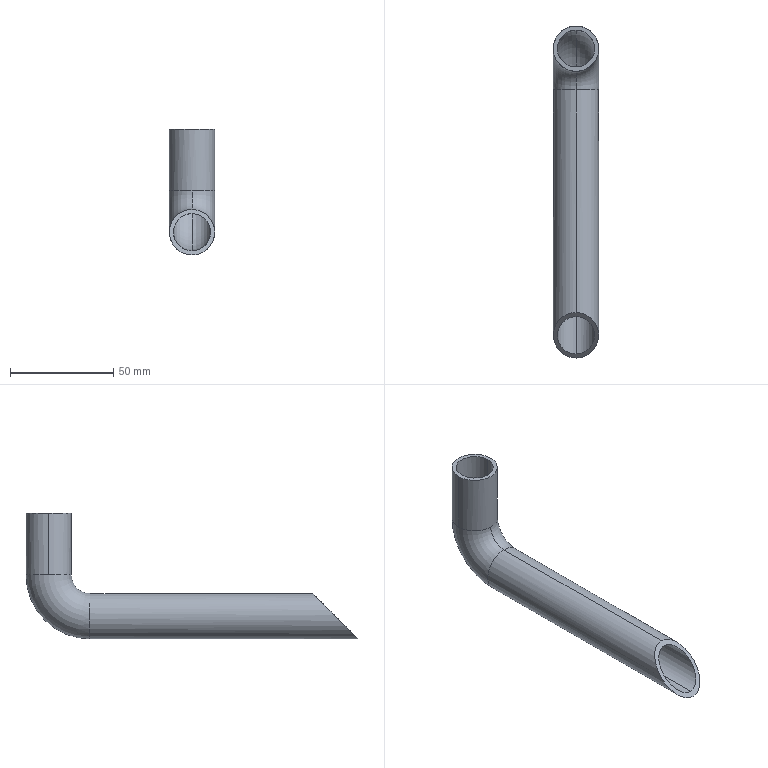Part | SolidWorks | features ICE 1, Sweep 1 | 1 solid | 14 faces | box 22 x 161 x 61 mm | volume 22672 mm3 | cylinder 8 | torus 4 | plane 2 | commonest cylinder face diameters 18 x4 22 x4
STEP:
#1=CARTESIAN_POINT('',(9.,0.,-30.));
#2=VERTEX_POINT('',#1);
#3=CARTESIAN_POINT('',(0.,9.,-30.));
#4=VERTEX_POINT('',#3);
#5=CARTESIAN_POINT('',(0.,0.,-30.));
#6=DIRECTION('',(0.,0.,1.));
#7=DIRECTION('',(1.,0.,0.));
#8=AXIS2_PLACEMENT_3D('',#5,#6,#7);
#9=CIRCLE('',#8,9.);
#10=EDGE_CURVE('',#2,#4,#9,.T.);
#11=ORIENTED_EDGE('',*,*,#10,.T.);
#12=CARTESIAN_POINT('',(0.,-20.,-59.));
#13=VERTEX_POINT('',#12);
#14=CARTESIAN_POINT('',(0.,-20.,-30.));
#15=DIRECTION('',(-1.,0.,0.));
#16=DIRECTION('',(0.,0.,1.));
#17=AXIS2_PLACEMENT_3D('',#14,#15,#16);
#18=CIRCLE('',#17,29.);
#19=EDGE_CURVE('',#4,#13,#18,.T.);
#20=ORIENTED_EDGE('',*,*,#19,.T.);
#21=CARTESIAN_POINT('',(0.,-20.,-41.));
#22=VERTEX_POINT('',#21);
#23=CARTESIAN_POINT('',(0.,-20.,-50.));
#24=DIRECTION('',(0.,1.,0.));
#25=DIRECTION('',(1.,0.,0.));
#26=AXIS2_PLACEMENT_3D('',#23,#24,#25);
#27=CIRCLE('',#26,9.);
#28=EDGE_CURVE('',#22,#13,#27,.T.);
#29=ORIENTED_EDGE('',*,*,#28,.F.);
#30=CARTESIAN_POINT('',(0.,-9.,-30.));
#31=VERTEX_POINT('',#30);
#32=CARTESIAN_POINT('',(0.,-20.,-30.));
#33=DIRECTION('',(-1.,0.,0.));
#34=DIRECTION('',(0.,0.,1.));
#35=AXIS2_PLACEMENT_3D('',#32,#33,#34);
#36=CIRCLE('',#35,11.);
#37=EDGE_CURVE('',#31,#22,#36,.T.);
#38=ORIENTED_EDGE('',*,*,#37,.F.);
#39=CARTESIAN_POINT('',(0.,0.,-30.));
#40=DIRECTION('',(0.,0.,1.));
#41=DIRECTION('',(1.,0.,0.));
#42=AXIS2_PLACEMENT_3D('',#39,#40,#41);
#43=CIRCLE('',#42,9.);
#44=EDGE_CURVE('',#31,#2,#43,.T.);
#45=ORIENTED_EDGE('',*,*,#44,.T.);
#46=EDGE_LOOP('',(#11,#20,#29,#38,#45));
#47=FACE_OUTER_BOUND('',#46,.T.);
#48=CARTESIAN_POINT('',(0.,-20.,-30.));
#49=DIRECTION('',(-1.,0.,0.));
#50=DIRECTION('',(0.,0.,1.));
#51=AXIS2_PLACEMENT_3D('',#48,#49,#50);
#52=TOROIDAL_SURFACE('',#51,20.,9.);
#53=ADVANCED_FACE('',(#47),#52,.F.);
#54=CARTESIAN_POINT('',(0.,11.,-30.));
#55=VERTEX_POINT('',#54);
#56=CARTESIAN_POINT('',(-11.,0.,-30.));
#57=VERTEX_POINT('',#56);
#58=CARTESIAN_POINT('',(0.,0.,-30.));
#59=DIRECTION('',(0.,0.,1.));
#60=DIRECTION('',(1.,0.,0.));
#61=AXIS2_PLACEMENT_3D('',#58,#59,#60);
#62=CIRCLE('',#61,11.);
#63=EDGE_CURVE('',#55,#57,#62,.T.);
#64=ORIENTED_EDGE('',*,*,#63,.F.);
#65=CARTESIAN_POINT('',(0.,-20.,-61.));
#66=VERTEX_POINT('',#65);
#67=CARTESIAN_POINT('',(0.,-20.,-30.));
#68=DIRECTION('',(-1.,0.,0.));
#69=DIRECTION('',(0.,0.,1.));
#70=AXIS2_PLACEMENT_3D('',#67,#68,#69);
#71=CIRCLE('',#70,31.);
#72=EDGE_CURVE('',#55,#66,#71,.T.);
#73=ORIENTED_EDGE('',*,*,#72,.T.);
#74=CARTESIAN_POINT('',(0.,-20.,-39.));
#75=VERTEX_POINT('',#74);
#76=CARTESIAN_POINT('',(0.,-20.,-50.));
#77=DIRECTION('',(0.,1.,0.));
#78=DIRECTION('',(1.,0.,0.));
#79=AXIS2_PLACEMENT_3D('',#76,#77,#78);
#80=CIRCLE('',#79,11.);
#81=EDGE_CURVE('',#66,#75,#80,.T.);
#82=ORIENTED_EDGE('',*,*,#81,.T.);
#83=CARTESIAN_POINT('',(0.,-11.,-30.));
#84=VERTEX_POINT('',#83);
#85=CARTESIAN_POINT('',(0.,-20.,-30.));
#86=DIRECTION('',(-1.,0.,0.));
#87=DIRECTION('',(0.,0.,1.));
#88=AXIS2_PLACEMENT_3D('',#85,#86,#87);
#89=CIRCLE('',#88,9.);
#90=EDGE_CURVE('',#84,#75,#89,.T.);
#91=ORIENTED_EDGE('',*,*,#90,.F.);
#92=CARTESIAN_POINT('',(0.,0.,-30.));
#93=DIRECTION('',(0.,0.,1.));
#94=DIRECTION('',(1.,0.,0.));
#95=AXIS2_PLACEMENT_3D('',#92,#93,#94);
#96=CIRCLE('',#95,11.);
#97=EDGE_CURVE('',#57,#84,#96,.T.);
#98=ORIENTED_EDGE('',*,*,#97,.F.);
#99=EDGE_LOOP('',(#64,#73,#82,#91,#98));
#100=FACE_OUTER_BOUND('',#99,.T.);
#101=CARTESIAN_POINT('',(0.,-20.,-30.));
#102=DIRECTION('',(-1.,0.,0.));
#103=DIRECTION('',(0.,0.,1.));
#104=AXIS2_PLACEMENT_3D('',#101,#102,#103);
#105=TOROIDAL_SURFACE('',#104,20.,11.);
#106=ADVANCED_FACE('',(#100),#105,.T.);
#107=CARTESIAN_POINT('',(11.,0.,-30.));
#108=VERTEX_POINT('',#107);
#109=CARTESIAN_POINT('',(0.,0.,-30.));
#110=DIRECTION('',(0.,0.,1.));
#111=DIRECTION('',(1.,0.,0.));
#112=AXIS2_PLACEMENT_3D('',#109,#110,#111);
#113=CIRCLE('',#112,11.);
#114=EDGE_CURVE('',#108,#55,#113,.T.);
#115=ORIENTED_EDGE('',*,*,#114,.T.);
#116=ORIENTED_EDGE('',*,*,#63,.T.);
#117=CARTESIAN_POINT('',(-11.,0.,0.));
#118=VERTEX_POINT('',#117);
#119=CARTESIAN_POINT('',(-11.,0.,-30.));
#120=DIRECTION('',(0.,0.,1.));
#121=VECTOR('',#120,1000.);
#122=LINE('',#119,#121);
#123=EDGE_CURVE('',#57,#118,#122,.T.);
#124=ORIENTED_EDGE('',*,*,#123,.T.);
#125=CARTESIAN_POINT('',(11.,0.,0.));
#126=VERTEX_POINT('',#125);
#127=CARTESIAN_POINT('',(0.,0.,0.));
#128=DIRECTION('',(0.,0.,1.));
#129=DIRECTION('',(1.,0.,0.));
#130=AXIS2_PLACEMENT_3D('',#127,#128,#129);
#131=CIRCLE('',#130,11.);
#132=EDGE_CURVE('',#126,#118,#131,.T.);
#133=ORIENTED_EDGE('',*,*,#132,.F.);
#134=CARTESIAN_POINT('',(11.,0.,-30.));
#135=DIRECTION('',(0.,0.,1.));
#136=VECTOR('',#135,1000.);
#137=LINE('',#134,#136);
#138=EDGE_CURVE('',#108,#126,#137,.T.);
#139=ORIENTED_EDGE('',*,*,#138,.F.);
#140=EDGE_LOOP('',(#115,#116,#124,#133,#139));
#141=FACE_OUTER_BOUND('',#140,.T.);
#142=CARTESIAN_POINT('',(0.,0.,-30.));
#143=DIRECTION('',(0.,0.,1.));
#144=DIRECTION('',(1.,0.,0.));
#145=AXIS2_PLACEMENT_3D('',#142,#143,#144);
#146=CYLINDRICAL_SURFACE('',#145,11.);
#147=ADVANCED_FACE('',(#141),#146,.T.);
#148=CARTESIAN_POINT('',(-9.,0.,-30.));
#149=VERTEX_POINT('',#148);
#150=CARTESIAN_POINT('',(0.,0.,-30.));
#151=DIRECTION('',(0.,0.,1.));
#152=DIRECTION('',(1.,0.,0.));
#153=AXIS2_PLACEMENT_3D('',#150,#151,#152);
#154=CIRCLE('',#153,9.);
#155=EDGE_CURVE('',#149,#31,#154,.T.);
#156=ORIENTED_EDGE('',*,*,#155,.F.);
#157=CARTESIAN_POINT('',(-9.,0.,0.));
#158=VERTEX_POINT('',#157);
#159=CARTESIAN_POINT('',(-9.,0.,-30.));
#160=DIRECTION('',(0.,0.,1.));
#161=VECTOR('',#160,1000.);
#162=LINE('',#159,#161);
#163=EDGE_CURVE('',#149,#158,#162,.T.);
#164=ORIENTED_EDGE('',*,*,#163,.T.);
#165=CARTESIAN_POINT('',(9.,0.,0.));
#166=VERTEX_POINT('',#165);
#167=CARTESIAN_POINT('',(0.,0.,0.));
#168=DIRECTION('',(0.,0.,1.));
#169=DIRECTION('',(1.,0.,0.));
#170=AXIS2_PLACEMENT_3D('',#167,#168,#169);
#171=CIRCLE('',#170,9.);
#172=EDGE_CURVE('',#158,#166,#171,.T.);
#173=ORIENTED_EDGE('',*,*,#172,.T.);
#174=CARTESIAN_POINT('',(9.,0.,-30.));
#175=DIRECTION('',(0.,0.,1.));
#176=VECTOR('',#175,1000.);
#177=LINE('',#174,#176);
#178=EDGE_CURVE('',#2,#166,#177,.T.);
#179=ORIENTED_EDGE('',*,*,#178,.F.);
#180=ORIENTED_EDGE('',*,*,#44,.F.);
#181=EDGE_LOOP('',(#156,#164,#173,#179,#180));
#182=FACE_OUTER_BOUND('',#181,.T.);
#183=CARTESIAN_POINT('',(0.,0.,-30.));
#184=DIRECTION('',(0.,0.,1.));
#185=DIRECTION('',(1.,0.,0.));
#186=AXIS2_PLACEMENT_3D('',#183,#184,#185);
#187=CYLINDRICAL_SURFACE('',#186,9.);
#188=ADVANCED_FACE('',(#182),#187,.F.);
#189=CARTESIAN_POINT('',(0.,-20.,-50.));
#190=DIRECTION('',(0.,1.,0.));
#191=DIRECTION('',(1.,0.,0.));
#192=AXIS2_PLACEMENT_3D('',#189,#190,#191);
#193=CIRCLE('',#192,9.);
#194=EDGE_CURVE('',#13,#22,#193,.T.);
#195=ORIENTED_EDGE('',*,*,#194,.T.);
#196=CARTESIAN_POINT('',(0.,-130.,-41.));
#197=VERTEX_POINT('',#196);
#198=CARTESIAN_POINT('',(0.,-20.,-41.));
#199=DIRECTION('',(0.,-1.,0.));
#200=VECTOR('',#199,1000.);
#201=LINE('',#198,#200);
#202=EDGE_CURVE('',#22,#197,#201,.T.);
#203=ORIENTED_EDGE('',*,*,#202,.T.);
#204=CARTESIAN_POINT('',(0.,-148.,-59.));
#205=VERTEX_POINT('',#204);
#206=CARTESIAN_POINT('',(0.,-148.,-59.));
#207=CARTESIAN_POINT('',(-18.,-148.,-59.));
#208=CARTESIAN_POINT('',(-18.,-130.,-41.));
#209=CARTESIAN_POINT('',(0.,-130.,-41.));
#210=(BOUNDED_CURVE()B_SPLINE_CURVE(3,(#206,#207,#208,#209),.UNSPECIFIED.,.F.,.T.)B_SPLINE_CURVE_WITH_KNOTS((4,4),(0.,3.142),.UNSPECIFIED.)CURVE()GEOMETRIC_REPRESENTATION_ITEM()RATIONAL_B_SPLINE_CURVE((1.,0.3333,0.3333,1.))REPRESENTATION_ITEM(''));
#211=EDGE_CURVE('',#205,#197,#210,.T.);
#212=ORIENTED_EDGE('',*,*,#211,.F.);
#213=CARTESIAN_POINT('',(0.,-20.,-59.));
#214=DIRECTION('',(0.,-1.,0.));
#215=VECTOR('',#214,1000.);
#216=LINE('',#213,#215);
#217=EDGE_CURVE('',#13,#205,#216,.T.);
#218=ORIENTED_EDGE('',*,*,#217,.F.);
#219=EDGE_LOOP('',(#195,#203,#212,#218));
#220=FACE_OUTER_BOUND('',#219,.T.);
#221=CARTESIAN_POINT('',(0.,-20.,-50.));
#222=DIRECTION('',(0.,-1.,0.));
#223=DIRECTION('',(0.,0.,-1.));
#224=AXIS2_PLACEMENT_3D('',#221,#222,#223);
#225=CYLINDRICAL_SURFACE('',#224,9.);
#226=ADVANCED_FACE('',(#220),#225,.F.);
#227=CARTESIAN_POINT('',(0.,-20.,-50.));
#228=DIRECTION('',(0.,1.,0.));
#229=DIRECTION('',(1.,0.,0.));
#230=AXIS2_PLACEMENT_3D('',#227,#228,#229);
#231=CIRCLE('',#230,11.);
#232=EDGE_CURVE('',#75,#66,#231,.T.);
#233=ORIENTED_EDGE('',*,*,#232,.F.);
#234=CARTESIAN_POINT('',(0.,-128.,-39.));
#235=VERTEX_POINT('',#234);
#236=CARTESIAN_POINT('',(0.,-20.,-39.));
#237=DIRECTION('',(0.,-1.,0.));
#238=VECTOR('',#237,1000.);
#239=LINE('',#236,#238);
#240=EDGE_CURVE('',#75,#235,#239,.T.);
#241=ORIENTED_EDGE('',*,*,#240,.T.);
#242=CARTESIAN_POINT('',(0.,-150.,-61.));
#243=VERTEX_POINT('',#242);
#244=CARTESIAN_POINT('',(0.,-128.,-39.));
#245=CARTESIAN_POINT('',(22.,-128.,-39.));
#246=CARTESIAN_POINT('',(22.,-150.,-61.));
#247=CARTESIAN_POINT('',(0.,-150.,-61.));
#248=(BOUNDED_CURVE()B_SPLINE_CURVE(3,(#244,#245,#246,#247),.UNSPECIFIED.,.F.,.T.)B_SPLINE_CURVE_WITH_KNOTS((4,4),(3.142,6.283),.UNSPECIFIED.)CURVE()GEOMETRIC_REPRESENTATION_ITEM()RATIONAL_B_SPLINE_CURVE((1.,0.3333,0.3333,1.))REPRESENTATION_ITEM(''));
#249=EDGE_CURVE('',#235,#243,#248,.T.);
#250=ORIENTED_EDGE('',*,*,#249,.T.);
#251=CARTESIAN_POINT('',(0.,-20.,-61.));
#252=DIRECTION('',(0.,-1.,0.));
#253=VECTOR('',#252,1000.);
#254=LINE('',#251,#253);
#255=EDGE_CURVE('',#66,#243,#254,.T.);
#256=ORIENTED_EDGE('',*,*,#255,.F.);
#257=EDGE_LOOP('',(#233,#241,#250,#256));
#258=FACE_OUTER_BOUND('',#257,.T.);
#259=CARTESIAN_POINT('',(0.,-20.,-50.));
#260=DIRECTION('',(0.,-1.,0.));
#261=DIRECTION('',(0.,0.,-1.));
#262=AXIS2_PLACEMENT_3D('',#259,#260,#261);
#263=CYLINDRICAL_SURFACE('',#262,11.);
#264=ADVANCED_FACE('',(#258),#263,.T.);
#265=ORIENTED_EDGE('',*,*,#240,.F.);
#266=ORIENTED_EDGE('',*,*,#81,.F.);
#267=ORIENTED_EDGE('',*,*,#255,.T.);
#268=CARTESIAN_POINT('',(0.,-150.,-61.));
#269=CARTESIAN_POINT('',(-22.,-150.,-61.));
#270=CARTESIAN_POINT('',(-22.,-128.,-39.));
#271=CARTESIAN_POINT('',(0.,-128.,-39.));
#272=(BOUNDED_CURVE()B_SPLINE_CURVE(3,(#268,#269,#270,#271),.UNSPECIFIED.,.F.,.T.)B_SPLINE_CURVE_WITH_KNOTS((4,4),(0.,3.142),.UNSPECIFIED.)CURVE()GEOMETRIC_REPRESENTATION_ITEM()RATIONAL_B_SPLINE_CURVE((1.,0.3333,0.3333,1.))REPRESENTATION_ITEM(''));
#273=EDGE_CURVE('',#243,#235,#272,.T.);
#274=ORIENTED_EDGE('',*,*,#273,.T.);
#275=EDGE_LOOP('',(#265,#266,#267,#274));
#276=FACE_OUTER_BOUND('',#275,.T.);
#277=CARTESIAN_POINT('',(0.,-20.,-50.));
#278=DIRECTION('',(0.,-1.,0.));
#279=DIRECTION('',(0.,0.,-1.));
#280=AXIS2_PLACEMENT_3D('',#277,#278,#279);
#281=CYLINDRICAL_SURFACE('',#280,11.);
#282=ADVANCED_FACE('',(#276),#281,.T.);
#283=ORIENTED_EDGE('',*,*,#202,.F.);
#284=ORIENTED_EDGE('',*,*,#28,.T.);
#285=ORIENTED_EDGE('',*,*,#217,.T.);
#286=CARTESIAN_POINT('',(0.,-130.,-41.));
#287=CARTESIAN_POINT('',(18.,-130.,-41.));
#288=CARTESIAN_POINT('',(18.,-148.,-59.));
#289=CARTESIAN_POINT('',(0.,-148.,-59.));
#290=(BOUNDED_CURVE()B_SPLINE_CURVE(3,(#286,#287,#288,#289),.UNSPECIFIED.,.F.,.F.)B_SPLINE_CURVE_WITH_KNOTS((4,4),(3.142,6.283),.UNSPECIFIED.)CURVE()GEOMETRIC_REPRESENTATION_ITEM()RATIONAL_B_SPLINE_CURVE((1.,0.3333,0.3333,1.))REPRESENTATION_ITEM(''));
#291=EDGE_CURVE('',#197,#205,#290,.T.);
#292=ORIENTED_EDGE('',*,*,#291,.F.);
#293=EDGE_LOOP('',(#283,#284,#285,#292));
#294=FACE_OUTER_BOUND('',#293,.T.);
#295=CARTESIAN_POINT('',(0.,-20.,-50.));
#296=DIRECTION('',(0.,-1.,0.));
#297=DIRECTION('',(0.,0.,-1.));
#298=AXIS2_PLACEMENT_3D('',#295,#296,#297);
#299=CYLINDRICAL_SURFACE('',#298,9.);
#300=ADVANCED_FACE('',(#294),#299,.F.);
#301=ORIENTED_EDGE('',*,*,#72,.F.);
#302=ORIENTED_EDGE('',*,*,#114,.F.);
#303=CARTESIAN_POINT('',(0.,0.,-30.));
#304=DIRECTION('',(0.,0.,1.));
#305=DIRECTION('',(1.,0.,0.));
#306=AXIS2_PLACEMENT_3D('',#303,#304,#305);
#307=CIRCLE('',#306,11.);
#308=EDGE_CURVE('',#84,#108,#307,.T.);
#309=ORIENTED_EDGE('',*,*,#308,.F.);
#310=ORIENTED_EDGE('',*,*,#90,.T.);
#311=ORIENTED_EDGE('',*,*,#232,.T.);
#312=EDGE_LOOP('',(#301,#302,#309,#310,#311));
#313=FACE_OUTER_BOUND('',#312,.T.);
#314=CARTESIAN_POINT('',(0.,-20.,-30.));
#315=DIRECTION('',(-1.,0.,0.));
#316=DIRECTION('',(0.,0.,1.));
#317=AXIS2_PLACEMENT_3D('',#314,#315,#316);
#318=TOROIDAL_SURFACE('',#317,20.,11.);
#319=ADVANCED_FACE('',(#313),#318,.T.);
#320=ORIENTED_EDGE('',*,*,#19,.F.);
#321=CARTESIAN_POINT('',(0.,0.,-30.));
#322=DIRECTION('',(0.,0.,1.));
#323=DIRECTION('',(1.,0.,0.));
#324=AXIS2_PLACEMENT_3D('',#321,#322,#323);
#325=CIRCLE('',#324,9.);
#326=EDGE_CURVE('',#4,#149,#325,.T.);
#327=ORIENTED_EDGE('',*,*,#326,.T.);
#328=ORIENTED_EDGE('',*,*,#155,.T.);
#329=ORIENTED_EDGE('',*,*,#37,.T.);
#330=ORIENTED_EDGE('',*,*,#194,.F.);
#331=EDGE_LOOP('',(#320,#327,#328,#329,#330));
#332=FACE_OUTER_BOUND('',#331,.T.);
#333=CARTESIAN_POINT('',(0.,-20.,-30.));
#334=DIRECTION('',(-1.,0.,0.));
#335=DIRECTION('',(0.,0.,1.));
#336=AXIS2_PLACEMENT_3D('',#333,#334,#335);
#337=TOROIDAL_SURFACE('',#336,20.,9.);
#338=ADVANCED_FACE('',(#332),#337,.F.);
#339=ORIENTED_EDGE('',*,*,#163,.F.);
#340=ORIENTED_EDGE('',*,*,#326,.F.);
#341=ORIENTED_EDGE('',*,*,#10,.F.);
#342=ORIENTED_EDGE('',*,*,#178,.T.);
#343=CARTESIAN_POINT('',(0.,0.,0.));
#344=DIRECTION('',(0.,0.,1.));
#345=DIRECTION('',(1.,0.,0.));
#346=AXIS2_PLACEMENT_3D('',#343,#344,#345);
#347=CIRCLE('',#346,9.);
#348=EDGE_CURVE('',#166,#158,#347,.T.);
#349=ORIENTED_EDGE('',*,*,#348,.T.);
#350=EDGE_LOOP('',(#339,#340,#341,#342,#349));
#351=FACE_OUTER_BOUND('',#350,.T.);
#352=CARTESIAN_POINT('',(0.,0.,-30.));
#353=DIRECTION('',(0.,0.,1.));
#354=DIRECTION('',(1.,0.,0.));
#355=AXIS2_PLACEMENT_3D('',#352,#353,#354);
#356=CYLINDRICAL_SURFACE('',#355,9.);
#357=ADVANCED_FACE('',(#351),#356,.F.);
#358=ORIENTED_EDGE('',*,*,#123,.F.);
#359=ORIENTED_EDGE('',*,*,#97,.T.);
#360=ORIENTED_EDGE('',*,*,#308,.T.);
#361=ORIENTED_EDGE('',*,*,#138,.T.);
#362=CARTESIAN_POINT('',(0.,0.,0.));
#363=DIRECTION('',(0.,0.,1.));
#364=DIRECTION('',(1.,0.,0.));
#365=AXIS2_PLACEMENT_3D('',#362,#363,#364);
#366=CIRCLE('',#365,11.);
#367=EDGE_CURVE('',#118,#126,#366,.T.);
#368=ORIENTED_EDGE('',*,*,#367,.F.);
#369=EDGE_LOOP('',(#358,#359,#360,#361,#368));
#370=FACE_OUTER_BOUND('',#369,.T.);
#371=CARTESIAN_POINT('',(0.,0.,-30.));
#372=DIRECTION('',(0.,0.,1.));
#373=DIRECTION('',(1.,0.,0.));
#374=AXIS2_PLACEMENT_3D('',#371,#372,#373);
#375=CYLINDRICAL_SURFACE('',#374,11.);
#376=ADVANCED_FACE('',(#370),#375,.T.);
#377=ORIENTED_EDGE('',*,*,#348,.F.);
#378=ORIENTED_EDGE('',*,*,#172,.F.);
#379=EDGE_LOOP('',(#377,#378));
#380=FACE_BOUND('',#379,.T.);
#381=ORIENTED_EDGE('',*,*,#132,.T.);
#382=ORIENTED_EDGE('',*,*,#367,.T.);
#383=EDGE_LOOP('',(#381,#382));
#384=FACE_OUTER_BOUND('',#383,.T.);
#385=CARTESIAN_POINT('',(0.,0.,0.));
#386=DIRECTION('',(0.,0.,1.));
#387=DIRECTION('',(1.,0.,0.));
#388=AXIS2_PLACEMENT_3D('',#385,#386,#387);
#389=PLANE('',#388);
#390=ADVANCED_FACE('',(#380,#384),#389,.T.);
#391=ORIENTED_EDGE('',*,*,#211,.T.);
#392=ORIENTED_EDGE('',*,*,#291,.T.);
#393=EDGE_LOOP('',(#391,#392));
#394=FACE_BOUND('',#393,.T.);
#395=ORIENTED_EDGE('',*,*,#273,.F.);
#396=ORIENTED_EDGE('',*,*,#249,.F.);
#397=EDGE_LOOP('',(#395,#396));
#398=FACE_OUTER_BOUND('',#397,.T.);
#399=CARTESIAN_POINT('',(-25.,-150.,-61.));
#400=DIRECTION('',(0.,0.7071,-0.7071));
#401=DIRECTION('',(0.,0.7071,0.7071));
#402=AXIS2_PLACEMENT_3D('',#399,#400,#401);
#403=PLANE('',#402);
#404=ADVANCED_FACE('',(#394,#398),#403,.F.);
#405=CLOSED_SHELL('',(#53,#106,#147,#188,#226,#264,#282,#300,#319,#338,#357,#376,#390,#404));
#406=MANIFOLD_SOLID_BREP('',#405);
#407=CARTESIAN_POINT('',(0.,0.,0.));
#408=DIRECTION('',(0.,0.,1.));
#409=DIRECTION('',(1.,0.,0.));
#410=AXIS2_PLACEMENT_3D('',#407,#408,#409);
#411=(LENGTH_UNIT()NAMED_UNIT(*)SI_UNIT(.MILLI.,.METRE.));
#412=UNCERTAINTY_MEASURE_WITH_UNIT(LENGTH_MEASURE(0.00001),#411,'','');
#413=(NAMED_UNIT(*)PLANE_ANGLE_UNIT()SI_UNIT($,.RADIAN.));
#414=(NAMED_UNIT(*)SI_UNIT($,.STERADIAN.)SOLID_ANGLE_UNIT());
#415=(GEOMETRIC_REPRESENTATION_CONTEXT(3)GLOBAL_UNCERTAINTY_ASSIGNED_CONTEXT((#412))GLOBAL_UNIT_ASSIGNED_CONTEXT((#411,#413,#414))REPRESENTATION_CONTEXT('',''));
#416=ADVANCED_BREP_SHAPE_REPRESENTATION('',(#406,#410),#415);